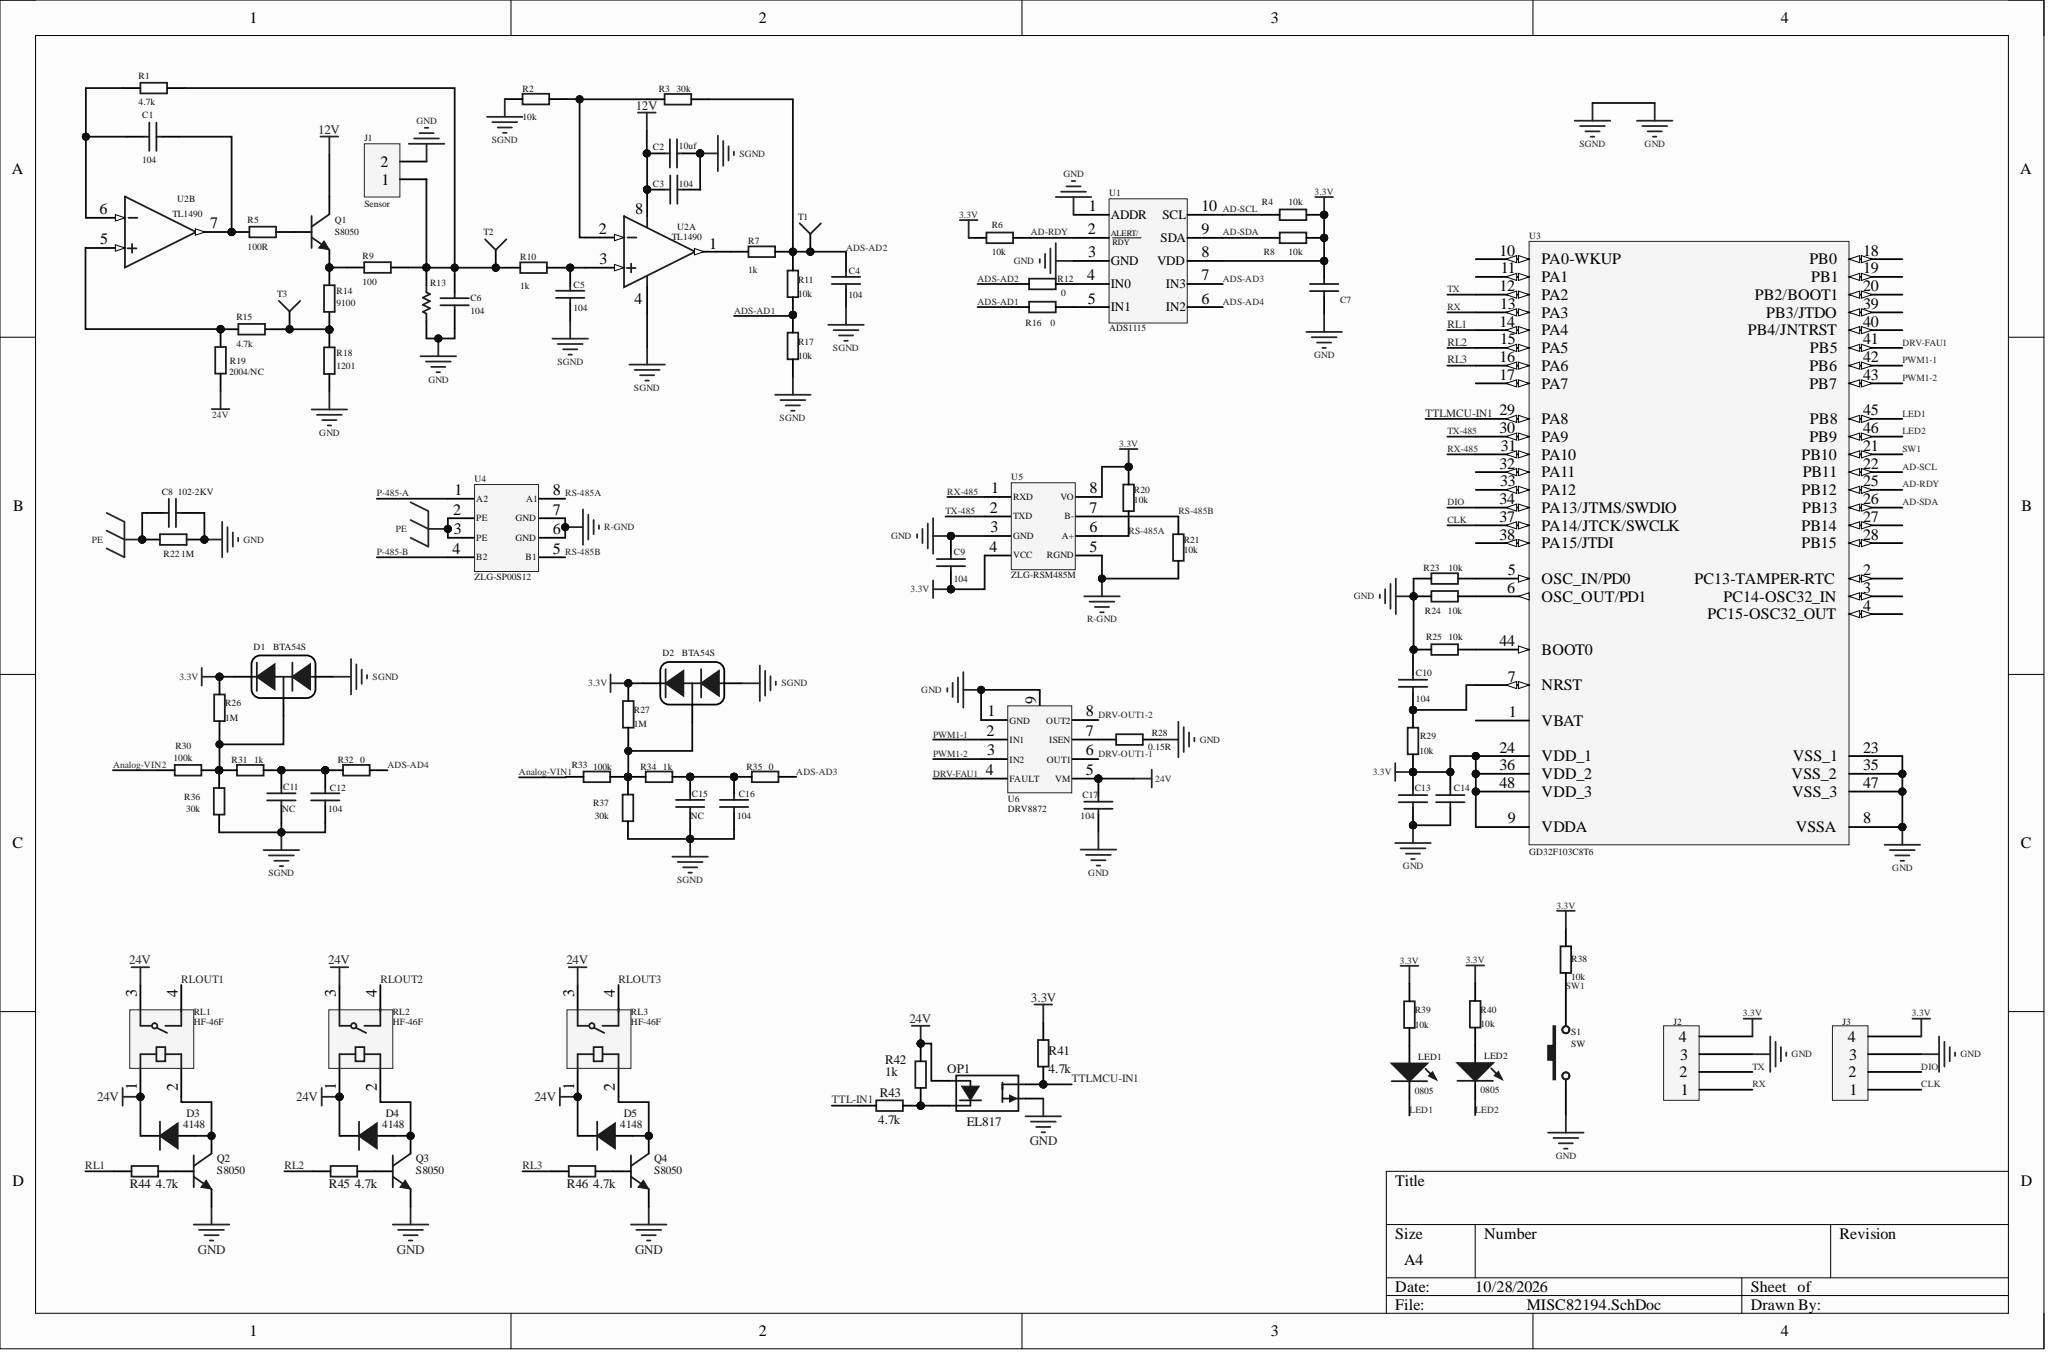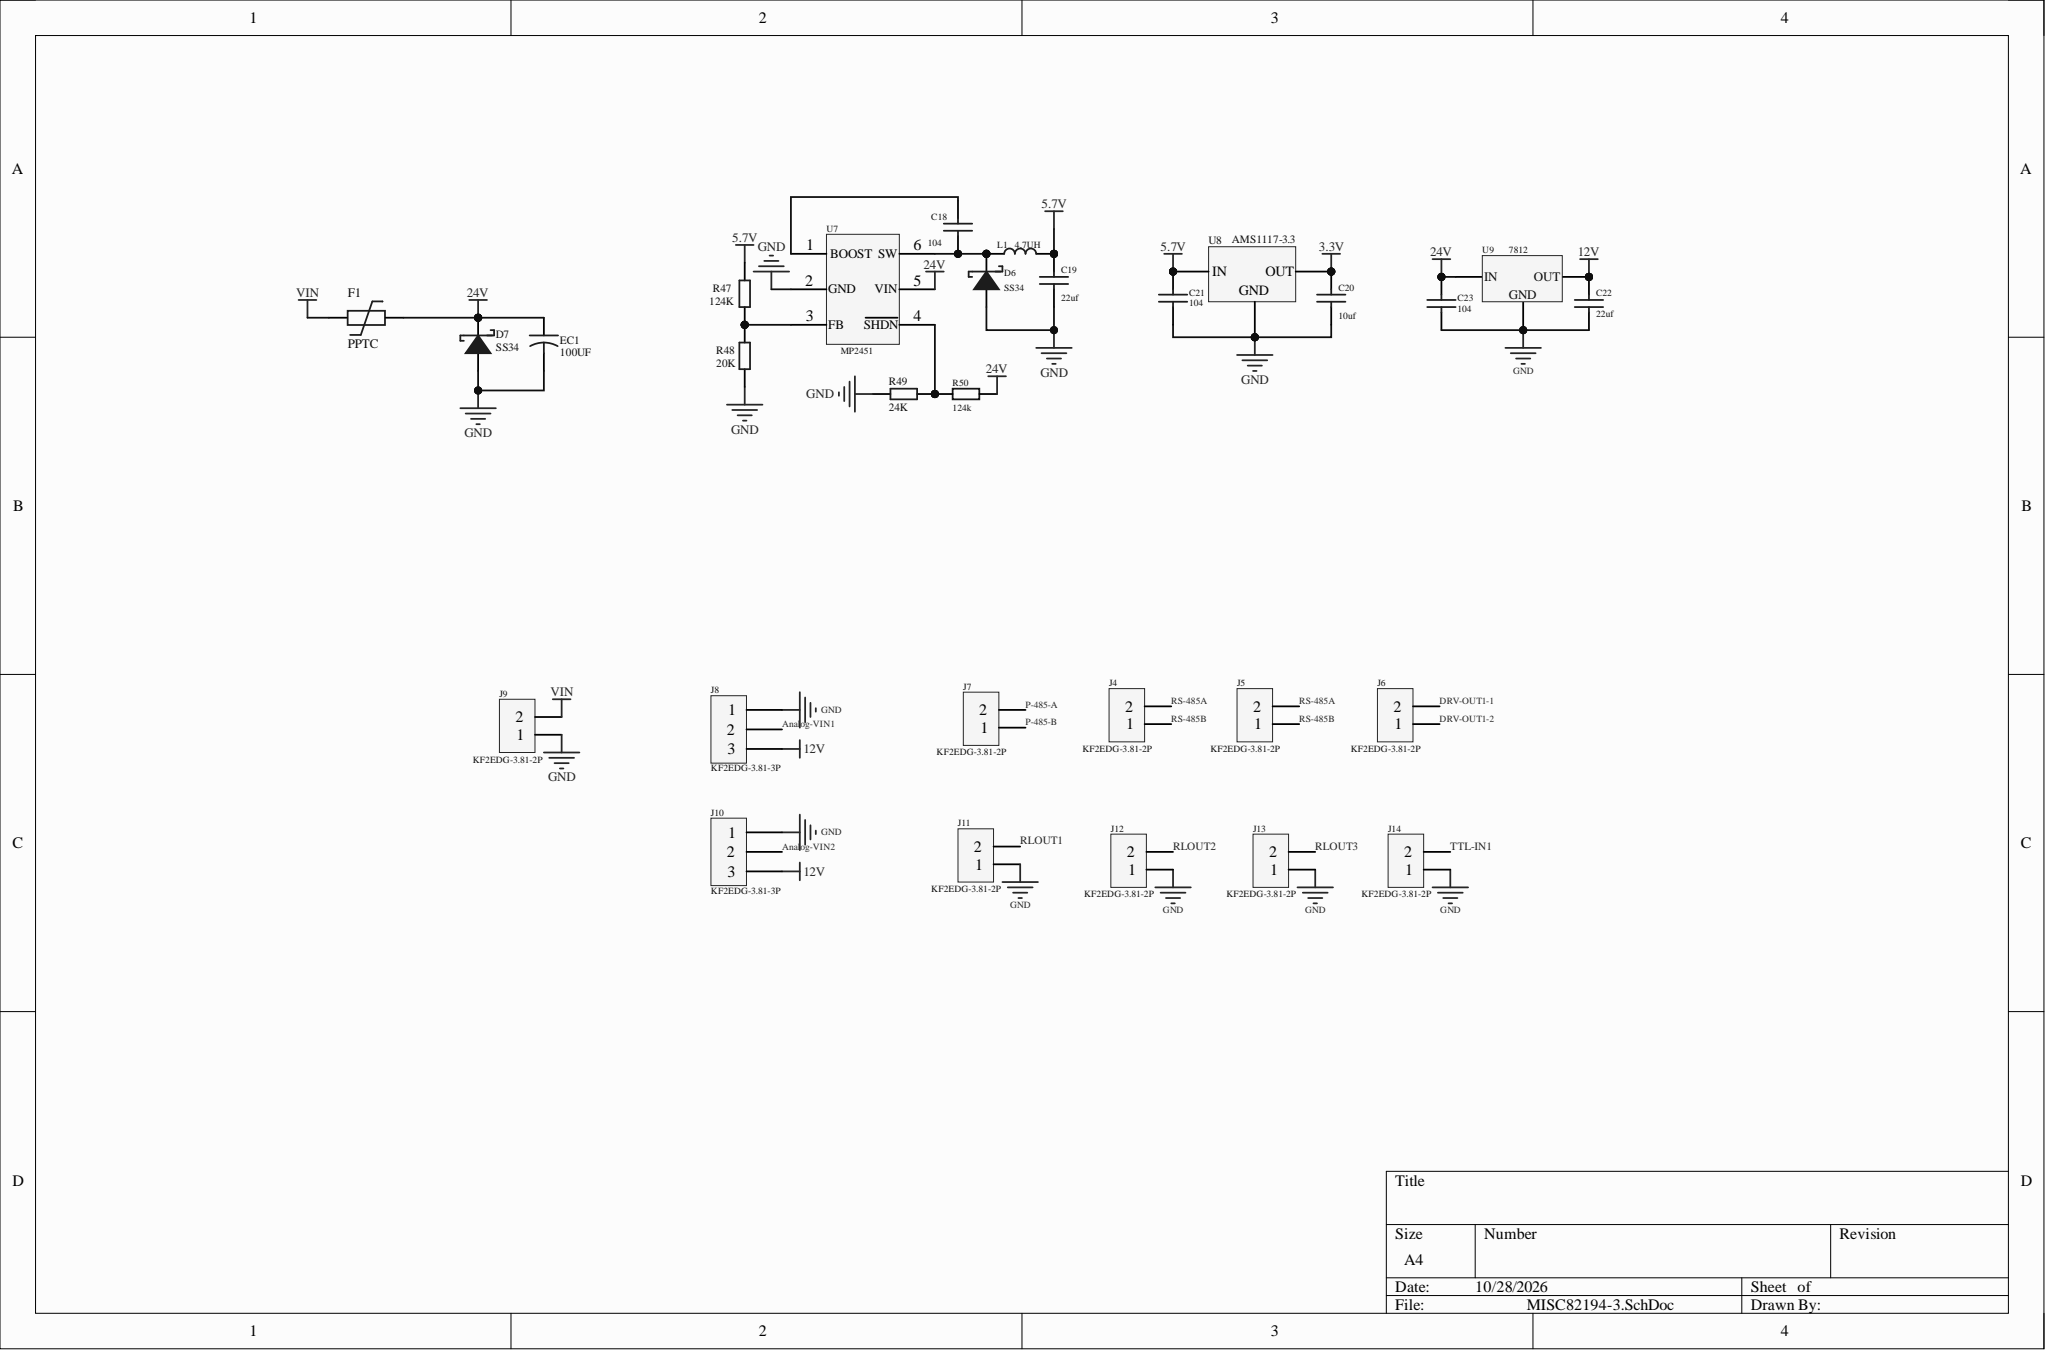Circuit board | Altium Designer | 120 parts | 77 nets
Bill of materials:
Comment,Description,Designator,Footprint,LibRef,Quantity
"104","","C1, C3, C4, C5, C6, C7, C9, C10, C12, C13, C14, C16, C17, C18, C21, C23","0805-C-I","Cap","16"
"10uf","","C2, C20","1206-C-I","Cap","2"
"102-2KV","","C8","1206-C-I","Cap","1"
"NC","","C11, C15","1206-C-I","Cap","2"
"22uf","","C19, C22","1206-C-I","Cap","2"
"BTA54S","","D1, D2","SOT23_L","DODI-II","2"
"4148","","D3, D4, D5","D1206","DIODE","3"
"SS34","","D6, D7","DO-SMA-I","DIODE-SBD","2"
"100UF","","EC1","C6.3X6.3","Cap Pol","1"
"PPTC","","F1","1210-F","FUSE-PTC","1"
"Sensor","","J1","3.81-2P-90","CON2","1"
"xh2.54","","J2, J3","CON4","CON4","2"
"KF2EDG-3.81-2P","","J4, J5, J6, J7, J9, J11, J12, J13, J14","3.81-2P-90","CON2","9"
"KF2EDG-3.81-3P","","J8, J10","3.81-3P-90","CON3","2"
"4.7UH","","L1","L-252012","INDUCTOR","1"
"0805","","LED1, LED2","LED[0805]","LED","2"
"EL817","","OP1","EL-817","Optocoupler","1"
"S8050","","Q1","SOT-89-3-1","BJT-NPN","1"
"S8050","","Q2, Q3, Q4","SOT23_L","BJT-NPN","3"
"4.7k","","R1, R15, R41, R43, R44, R45, R46","0805-R-I","R1","7"
"10k","","R2, R4, R6, R8, R11, R17, R20, R21, R23, R24, R25, R29, R38, R39, R40","0805-R-I","R1","15"
"30k","","R3, R36, R37","0805-R-I","R1","3"
"100R","","R5","0805-R-I","R1","1"
"1k","","R7, R10, R31, R34, R42","0805-R-I","R1","5"
"100","","R9","1206-R-I","R1","1"
"0","","R12, R16, R32, R35","0805-R-I","R1","4"
"","","R13","R[0805]","R","1"
"9100","","R14","0805-R-I","R1","1"
"1201","","R18","0805-R-I","R1","1"
"2004/NC","","R19","0805-R-I","R1","1"
"1M","","R22","1206-R-I","R1","1"
"1M","","R26, R27","0805-R-I","R1","2"
"0.15R","","R28","0805-R-I","R","1"
"100k","","R30, R33","0805-R-I","R1","2"
"124K","","R47, R50","0805-R-I","R1","2"
"20K","","R48","0805-R-I","R1","1"
"24K","","R49","0805-R-I","R1","1"
"HF-46F","","RL1, RL2, RL3","RY-HF46F","RELAY4","3"
"SW","","S1","KEY-3*6","Button","1"
"","","T1, T2, T3","TP-TEST","TP-TEST1","3"
"ADS1115","","U1","MSOP-10","ADS1115","1"
"TL1490","","U2","SO-8","OPAPM-2","1"
"GD32F103C8T6","STM32 ARM-based 32-bit MCU with 64 Kbytes Flash, 48-pin LQFP, Industrial Temperature","U3","LQFP48_N","STM32F103C8T6","1"
"ZLG-SP00S12","","U4","ZLG-SP00S12","ZLG-SP00S12","1"
"ZLG-RSM485M","","U5","ZLG-RSM485M","ZLG-RSM485M","1"
"DRV8872","","U6","SOP8-9","DRV8872","1"
"MP2451","","U7","SOT23-6","LT1933","1"
"AMS1117-3.3","","U8","SOT-223 - 3","AMS1117","1"
"7812","","U9","TO-252","LM7805","1"
Netlist (Protel format):
[
C1
0805-C-I
104



]
[
C2
1206-C-I
10uf



]
[
C3
0805-C-I
104



]
[
C4
0805-C-I
104



]
[
C5
0805-C-I
104



]
[
C6
0805-C-I
104



]
[
C7
0805-C-I
104



]
[
C8
1206-C-I
102-2KV



]
[
C9
0805-C-I
104



]
[
C10
0805-C-I
104



]
[
C11
1206-C-I
NC



]
[
C12
0805-C-I
104



]
[
C13
0805-C-I
104



]
[
C14
0805-C-I
104



]
[
C15
1206-C-I
NC



]
[
C16
0805-C-I
104



]
[
C17
0805-C-I
104



]
[
C18
0805-C-I
104



]
[
C19
1206-C-I
22uf



]
[
C20
1206-C-I
10uf



]
[
C21
0805-C-I
104



]
[
C22
1206-C-I
22uf



]
[
C23
0805-C-I
104



]
[
D1
SOT23_L
BTA54S



]
[
D2
SOT23_L
BTA54S



]
[
D3
D1206
4148



]
[
D4
D1206
4148



]
[
D5
D1206
4148



]
[
D6
DO-SMA-I
SS34



]
[
D7
DO-SMA-I
SS34



]
[
EC1
C6.3X6.3
100UF



]
[
F1
1210-F
PPTC



]
[
J1
3.81-2P-90
Sensor



]
[
J2
CON4
xh2.54



]
[
J3
CON4
xh2.54



]
[
J4
3.81-2P-90
KF2EDG-3.81-2P



]
[
J5
3.81-2P-90
KF2EDG-3.81-2P



]
[
J6
3.81-2P-90
KF2EDG-3.81-2P



]
[
J7
3.81-2P-90
KF2EDG-3.81-2P



]
[
J8
3.81-3P-90
KF2EDG-3.81-3P



]
[
J9
3.81-2P-90
KF2EDG-3.81-2P



]
[
J10
3.81-3P-90
KF2EDG-3.81-3P



]
[
J11
3.81-2P-90
KF2EDG-3.81-2P



]
[
J12
3.81-2P-90
KF2EDG-3.81-2P



]
[
J13
3.81-2P-90
KF2EDG-3.81-2P



]
[
J14
3.81-2P-90
KF2EDG-3.81-2P



]
[
L1
L-252012
4.7UH



]
[
LED1
LED[0805]
0805



]
[
LED2
LED[0805]
0805



]
[
OP1
EL-817
EL817



]
[
Q1
SOT-89-3-1
S8050



]
[
Q2
SOT23_L
S8050



]
[
Q3
SOT23_L
S8050



]
[
Q4
SOT23_L
S8050



]
[
R1
0805-R-I
4.7k



]
[
R2
0805-R-I
10k



]
[
R3
0805-R-I
30k



]
[
R4
0805-R-I
10k



]
[
R5
0805-R-I
100R



]
[
R6
0805-R-I
10k



]
[
R7
0805-R-I
1k



]
[
R8
0805-R-I
10k



]
[
R9
1206-R-I
100



]
[
R10
0805-R-I
1k



]
[
R11
0805-R-I
10k



]
[
R12
0805-R-I
0



]
[
R13
R[0805]




]
[
R14
0805-R-I
9100



]
[
R15
0805-R-I
4.7k



]
[
R16
0805-R-I
0



]
[
R17
0805-R-I
10k



]
[
R18
0805-R-I
1201



]
[
R19
0805-R-I
2004/NC



]
[
R20
0805-R-I
10k



]
[
R21
0805-R-I
10k



]
[
R22
1206-R-I
1M



]
[
R23
0805-R-I
10k



]
[
R24
0805-R-I
10k



]
[
R25
0805-R-I
10k



]
[
R26
0805-R-I
1M



]
[
R27
0805-R-I
1M



]
[
R28
0805-R-I
0.15R



]
[
R29
0805-R-I
10k



]
[
R30
0805-R-I
100k



]
[
R31
0805-R-I
1k



]
[
R32
0805-R-I
0



]
[
R33
0805-R-I
100k



]
[
R34
0805-R-I
1k



]
[
R35
0805-R-I
0



]
[
R36
0805-R-I
30k



]
[
R37
0805-R-I
30k



]
[
R38
0805-R-I
10k



]
[
R39
0805-R-I
10k



]
[
R40
0805-R-I
10k



]
[
R41
0805-R-I
4.7k



]
[
R42
0805-R-I
1k



]
[
R43
0805-R-I
4.7k



]
[
R44
0805-R-I
4.7k



]
[
R45
0805-R-I
4.7k



]
[
R46
0805-R-I
4.7k



]
[
R47
0805-R-I
124K



]
[
R48
0805-R-I
20K



]
[
R49
0805-R-I
24K



]
[
R50
0805-R-I
124k



]
[
RL1
RY-HF46F
HF-46F



]
[
RL2
RY-HF46F
HF-46F



]
[
RL3
RY-HF46F
HF-46F



]
[
S1
KEY-3*6
SW



]
[
T1
TP-TEST




]
[
T2
TP-TEST




]
[
T3
TP-TEST




]
[
U1
MSOP-10
ADS1115



]
[
U2
SO-8
TL1490



]
[
U3
LQFP48_N
GD32F103C8T6



]
[
U4
ZLG-SP00S12
ZLG-SP00S12



]
[
U5
ZLG-RSM485M
ZLG-RSM485M



]
[
U6
SOP8-9
DRV8872



]
[
U7
SOT23-6
MP2451



]
[
U8
SOT-223 - 3
AMS1117-3.3



]
[
U9
TO-252
7812



]
(
VIN
F1-1
J9-2
)
(
TX-485
U3-30
U5-2
)
(
TX
J2-2
U3-12
)
(
TTLMCU-IN1
OP1-4
R41-1
U3-29
)
(
TTL-IN1
J14-2
R43-1
)
(
SW1
R38-1
S1-2
U3-21
)
(
RX-485
U3-31
U5-1
)
(
RX
J2-1
U3-13
)
(
RS-485B
J4-1
J5-1
R21-2
U4-5
U5-7
)
(
RS-485A
J4-2
J5-2
R20-1
U4-8
U5-6
)
(
RLOUT3
J13-2
RL3-4
)
(
RLOUT2
J12-2
RL2-4
)
(
RLOUT1
J11-2
RL1-4
)
(
RL3
R46-2
U3-16
)
(
RL2
R45-2
U3-15
)
(
RL1
R44-2
U3-14
)
(
R-GND
R21-1
U4-6
U4-7
U5-5
)
(
PWM1-2
U3-43
U6-3
)
(
PWM1-1
U3-42
U6-2
)
(
PE
C8-1
R22-1
U4-2
U4-3
)
(
P-485-B
J7-1
U4-4
)
(
P-485-A
J7-2
U4-1
)
(
NetR49_2
R49-2
R50-1
U7-4
)
(
NetR47_2
R47-2
R48-1
U7-3
)
(
NetR28_2
R28-2
U6-7
)
(
NetR25_2
R25-2
U3-44
)
(
NetR24_1
R24-1
U3-6
)
(
NetR23_1
R23-1
U3-5
)
(
NetR16_2
R16-2
U1-5
)
(
NetR15_1
R15-1
R19-1
U2-5
)
(
NetR14_2
R14-2
R15-2
R18-1
T3-1
)
(
NetR12_2
R12-2
U1-4
)
(
NetR7_2
R7-2
U2-1
)
(
NetR2_1
R2-1
R3-2
U2-2
)
(
NetQ4_1
Q4-1
R46-1
)
(
NetQ3_1
Q3-1
R45-1
)
(
NetQ2_1
Q2-1
R44-1
)
(
NetQ1_2
Q1-2
R9-1
R14-1
)
(
NetQ1_1
Q1-1
R5-1
)
(
NetOP1_2
OP1-2
R42-1
R43-2
)
(
NetLED2_1
LED2-1
R40-1
)
(
NetLED1_1
LED1-1
R39-1
)
(
NetD5_1
D5-1
Q4-3
RL3-2
)
(
NetD4_1
D4-1
Q3-3
RL2-2
)
(
NetD3_1
D3-1
Q2-3
RL1-2
)
(
NetD2_3
D2-3
R27-1
R33-2
R34-1
R37-2
)
(
NetD1_3
D1-3
R26-1
R30-2
R31-1
R36-2
)
(
NetC18_2
C18-2
U7-1
)
(
NetC18_1
C18-1
D6-2
L1-1
U7-6
)
(
NetC15_2
C15-2
C16-2
R34-2
R35-1
)
(
NetC11_2
C11-2
C12-2
R31-2
R32-1
)
(
NetC10_1
C10-1
R29-1
U3-7
)
(
NetC6_1
C6-1
J1-1
R1-1
R9-2
R10-2
R13-2
T2-1
)
(
NetC5_2
C5-2
R10-1
U2-3
)
(
NetC1_2
C1-2
R1-2
U2-6
)
(
NetC1_1
C1-1
R5-2
U2-7
)
(
LED2
LED2-2
U3-46
)
(
LED1
LED1-2
U3-45
)
(
GND
C2-1
C3-1
C4-1
C5-1
C6-2
C7-1
C8-2
C9-2
C10-2
C11-1
C12-1
C13-1
C14-1
C15-1
C16-1
C17-1
C19-1
C20-1
C21-1
C22-1
C23-1
D1-1
D2-1
D6-1
D7-1
EC1-2
J1-2
J2-3
J3-3
J8-1
J9-1
J10-1
J11-1
J12-1
J13-1
J14-1
OP1-3
Q2-2
Q3-2
Q4-2
R2-2
R13-1
R17-2
R18-2
R22-2
R23-2
R24-2
R25-1
R28-1
R36-1
R37-1
R48-2
R49-1
S1-1
U1-1
U1-3
U2-4
U3-8
U3-23
U3-35
U3-47
U5-3
U6-1
U6-9
U7-2
U8-1
U9-2
)
(
DRV-OUT1-2
J6-1
U6-8
)
(
DRV-OUT1-1
J6-2
U6-6
)
(
DRV-FAU1
U3-41
U6-4
)
(
DIO
J3-2
U3-34
)
(
CLK
J3-1
U3-37
)
(
Analog-VIN2
J10-2
R30-1
)
(
Analog-VIN1
J8-2
R33-1
)
(
ADS-AD4
R32-2
U1-6
)
(
ADS-AD3
R35-2
U1-7
)
(
ADS-AD2
C4-2
R3-1
R7-1
R11-1
R12-1
T1-1
)
(
ADS-AD1
R11-2
R16-1
R17-1
)
(
AD-SDA
R8-1
U1-9
U3-26
)
(
AD-SCL
R4-1
U1-10
U3-22
)
(
AD-RDY
R6-2
U1-2
U3-25
)
(
24V
C17-2
C23-2
D3-2
D4-2
D5-2
D7-2
EC1-1
F1-2
OP1-1
R19-2
R42-2
R50-2
RL1-1
RL1-3
RL2-1
RL2-3
RL3-1
RL3-3
U6-5
U7-5
U9-1
)
(
12V
C2-2
C3-2
C22-2
J8-3
J10-3
Q1-3
U2-8
U9-3
)
(
5.7V
C19-2
C21-2
L1-2
R47-1
U8-3
)
(
3.3V
C7-2
C9-1
C13-2
C14-2
C20-2
D1-2
D2-2
J2-4
J3-4
R4-2
R6-1
R8-2
R20-2
R26-2
R27-2
R29-2
R38-2
R39-2
R40-2
R41-2
U1-8
U3-9
U3-24
U3-36
U3-48
U5-4
U5-8
U8-2
)